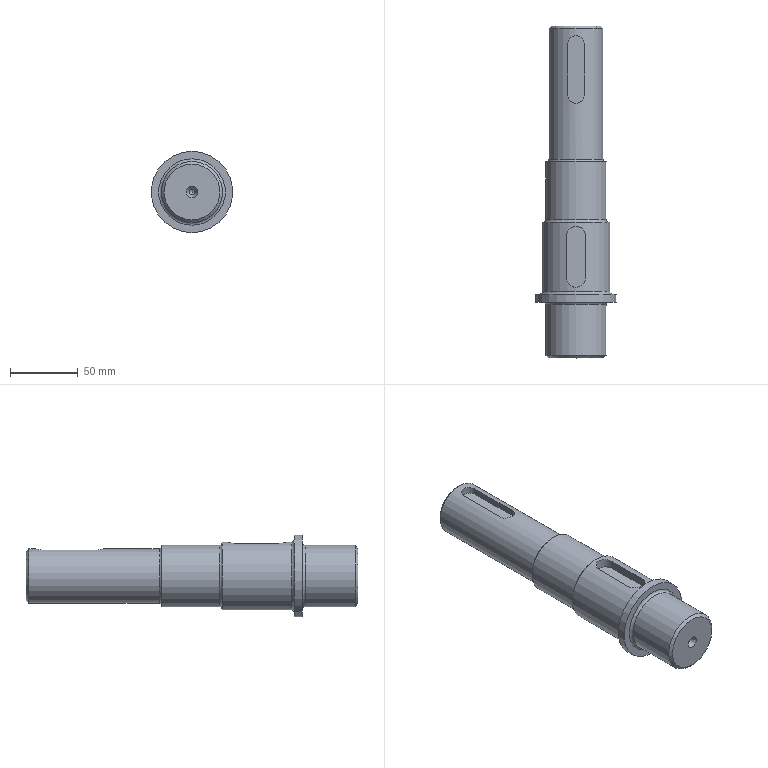Part | NX | features DATUM_CSYS 4, SKETCH 3, EXTRUDE 2, SWP104 1 | 1 solid | 33 faces | box 60 x 244.5 x 60 mm | volume 375385 mm3 | plane 12 | cylinder 11 | cone 6 | torus 4 | commonest cylinder face diameters 4 x2 12 x2 14 x2 45 x2 40 x1 50 x1
STEP:
#1=CARTESIAN_POINT('',(0.,242.5,-20.));
#2=VERTEX_POINT('',#1);
#3=CARTESIAN_POINT('',(0.,242.5,0.));
#4=DIRECTION('',(0.,-1.,0.));
#5=DIRECTION('',(0.,0.,-1.));
#6=AXIS2_PLACEMENT_3D('',#3,#4,#5);
#7=CIRCLE('',#6,20.);
#8=EDGE_CURVE('',#2,#2,#7,.T.);
#9=ORIENTED_EDGE('',*,*,#8,.T.);
#10=EDGE_LOOP('',(#9));
#11=FACE_BOUND('',#10,.T.);
#12=CARTESIAN_POINT('',(0.,146.5,-20.));
#13=VERTEX_POINT('',#12);
#14=CARTESIAN_POINT('',(0.,146.5,0.));
#15=DIRECTION('',(0.,-1.,0.));
#16=DIRECTION('',(0.,0.,-1.));
#17=AXIS2_PLACEMENT_3D('',#14,#15,#16);
#18=CIRCLE('',#17,20.);
#19=EDGE_CURVE('',#13,#13,#18,.T.);
#20=ORIENTED_EDGE('',*,*,#19,.F.);
#21=EDGE_LOOP('',(#20));
#22=FACE_BOUND('',#21,.T.);
#23=CARTESIAN_POINT('',(6.,193.5,19.079));
#24=VERTEX_POINT('',#23);
#25=CARTESIAN_POINT('',(-6.,193.5,19.079));
#26=VERTEX_POINT('',#25);
#27=CARTESIAN_POINT('',(6.,193.5,19.079));
#28=CARTESIAN_POINT('',(6.,191.905,19.079));
#29=CARTESIAN_POINT('',(4.699,188.813,19.55));
#30=CARTESIAN_POINT('',(0.009548,186.844,20.225));
#31=CARTESIAN_POINT('',(-4.702,188.81,19.551));
#32=CARTESIAN_POINT('',(-6.,191.905,19.079));
#33=CARTESIAN_POINT('',(-6.,193.5,19.079));
#34=B_SPLINE_CURVE_WITH_KNOTS('',3,(#27,#28,#29,#30,#31,#32,#33),.UNSPECIFIED.,.F.,.F.,(4,1,1,1,4),(0.,0.004715,0.009431,0.01415,0.01886),.UNSPECIFIED.);
#35=EDGE_CURVE('',#24,#26,#34,.T.);
#36=ORIENTED_EDGE('',*,*,#35,.T.);
#37=CARTESIAN_POINT('',(-6.,231.5,19.079));
#38=VERTEX_POINT('',#37);
#39=CARTESIAN_POINT('',(-6.,122.25,19.079));
#40=DIRECTION('',(0.,-1.,0.));
#41=VECTOR('',#40,1000.);
#42=LINE('',#39,#41);
#43=EDGE_CURVE('',#26,#38,#42,.F.);
#44=ORIENTED_EDGE('',*,*,#43,.T.);
#45=CARTESIAN_POINT('',(6.,231.5,19.079));
#46=VERTEX_POINT('',#45);
#47=CARTESIAN_POINT('',(-6.,231.5,19.079));
#48=CARTESIAN_POINT('',(-6.,233.095,19.079));
#49=CARTESIAN_POINT('',(-4.699,236.187,19.55));
#50=CARTESIAN_POINT('',(-0.009548,238.156,20.225));
#51=CARTESIAN_POINT('',(4.702,236.19,19.551));
#52=CARTESIAN_POINT('',(6.,233.095,19.079));
#53=CARTESIAN_POINT('',(6.,231.5,19.079));
#54=B_SPLINE_CURVE_WITH_KNOTS('',3,(#47,#48,#49,#50,#51,#52,#53),.UNSPECIFIED.,.F.,.F.,(4,1,1,1,4),(0.,0.004715,0.009431,0.01415,0.01886),.UNSPECIFIED.);
#55=EDGE_CURVE('',#38,#46,#54,.T.);
#56=ORIENTED_EDGE('',*,*,#55,.T.);
#57=CARTESIAN_POINT('',(6.,122.25,19.079));
#58=DIRECTION('',(0.,-1.,0.));
#59=VECTOR('',#58,1000.);
#60=LINE('',#57,#59);
#61=EDGE_CURVE('',#46,#24,#60,.T.);
#62=ORIENTED_EDGE('',*,*,#61,.T.);
#63=EDGE_LOOP('',(#36,#44,#56,#62));
#64=FACE_BOUND('',#63,.T.);
#65=CARTESIAN_POINT('',(0.,122.25,0.));
#66=DIRECTION('',(0.,-1.,0.));
#67=DIRECTION('',(0.,0.,-1.));
#68=AXIS2_PLACEMENT_3D('',#65,#66,#67);
#69=CYLINDRICAL_SURFACE('',#68,20.);
#70=ADVANCED_FACE('',(#11,#22,#64),#69,.T.);
#71=CARTESIAN_POINT('',(0.,100.,-25.));
#72=VERTEX_POINT('',#71);
#73=CARTESIAN_POINT('',(0.,100.,0.));
#74=DIRECTION('',(0.,-1.,0.));
#75=DIRECTION('',(0.,0.,-1.));
#76=AXIS2_PLACEMENT_3D('',#73,#74,#75);
#77=CIRCLE('',#76,25.);
#78=EDGE_CURVE('',#72,#72,#77,.T.);
#79=ORIENTED_EDGE('',*,*,#78,.T.);
#80=EDGE_LOOP('',(#79));
#81=FACE_BOUND('',#80,.T.);
#82=CARTESIAN_POINT('',(0.,49.,-25.));
#83=VERTEX_POINT('',#82);
#84=CARTESIAN_POINT('',(0.,49.,0.));
#85=DIRECTION('',(0.,-1.,0.));
#86=DIRECTION('',(0.,0.,-1.));
#87=AXIS2_PLACEMENT_3D('',#84,#85,#86);
#88=CIRCLE('',#87,25.);
#89=EDGE_CURVE('',#83,#83,#88,.T.);
#90=ORIENTED_EDGE('',*,*,#89,.F.);
#91=EDGE_LOOP('',(#90));
#92=FACE_BOUND('',#91,.T.);
#93=CARTESIAN_POINT('',(7.,59.,24.));
#94=VERTEX_POINT('',#93);
#95=CARTESIAN_POINT('',(-7.,59.,24.));
#96=VERTEX_POINT('',#95);
#97=CARTESIAN_POINT('',(7.,59.,24.));
#98=CARTESIAN_POINT('',(7.,57.141,24.));
#99=CARTESIAN_POINT('',(5.483,53.53,24.51));
#100=CARTESIAN_POINT('',(0.01059,51.236,25.245));
#101=CARTESIAN_POINT('',(-5.485,53.527,24.511));
#102=CARTESIAN_POINT('',(-7.,57.14,24.));
#103=CARTESIAN_POINT('',(-7.,59.,24.));
#104=B_SPLINE_CURVE_WITH_KNOTS('',3,(#97,#98,#99,#100,#101,#102,#103),.UNSPECIFIED.,.F.,.F.,(4,1,1,1,4),(0.,0.005497,0.01099,0.01649,0.02199),.UNSPECIFIED.);
#105=EDGE_CURVE('',#94,#96,#104,.T.);
#106=ORIENTED_EDGE('',*,*,#105,.T.);
#107=CARTESIAN_POINT('',(-7.,90.,24.));
#108=VERTEX_POINT('',#107);
#109=CARTESIAN_POINT('',(-7.,122.25,24.));
#110=DIRECTION('',(0.,-1.,0.));
#111=VECTOR('',#110,1000.);
#112=LINE('',#109,#111);
#113=EDGE_CURVE('',#96,#108,#112,.F.);
#114=ORIENTED_EDGE('',*,*,#113,.T.);
#115=CARTESIAN_POINT('',(7.,90.,24.));
#116=VERTEX_POINT('',#115);
#117=CARTESIAN_POINT('',(-7.,90.,24.));
#118=CARTESIAN_POINT('',(-7.,91.859,24.));
#119=CARTESIAN_POINT('',(-5.483,95.47,24.51));
#120=CARTESIAN_POINT('',(-0.01059,97.764,25.245));
#121=CARTESIAN_POINT('',(5.485,95.473,24.511));
#122=CARTESIAN_POINT('',(7.,91.86,24.));
#123=CARTESIAN_POINT('',(7.,90.,24.));
#124=B_SPLINE_CURVE_WITH_KNOTS('',3,(#117,#118,#119,#120,#121,#122,#123),.UNSPECIFIED.,.F.,.F.,(4,1,1,1,4),(0.,0.005497,0.01099,0.01649,0.02199),.UNSPECIFIED.);
#125=EDGE_CURVE('',#108,#116,#124,.T.);
#126=ORIENTED_EDGE('',*,*,#125,.T.);
#127=CARTESIAN_POINT('',(7.,122.25,24.));
#128=DIRECTION('',(0.,-1.,0.));
#129=VECTOR('',#128,1000.);
#130=LINE('',#127,#129);
#131=EDGE_CURVE('',#116,#94,#130,.T.);
#132=ORIENTED_EDGE('',*,*,#131,.T.);
#133=EDGE_LOOP('',(#106,#114,#126,#132));
#134=FACE_BOUND('',#133,.T.);
#135=CARTESIAN_POINT('',(0.,122.25,0.));
#136=DIRECTION('',(0.,-1.,0.));
#137=DIRECTION('',(0.,0.,-1.));
#138=AXIS2_PLACEMENT_3D('',#135,#136,#137);
#139=CYLINDRICAL_SURFACE('',#138,25.);
#140=ADVANCED_FACE('',(#81,#92,#134),#139,.T.);
#141=CARTESIAN_POINT('',(0.,0.,-4.309));
#142=VERTEX_POINT('',#141);
#143=CARTESIAN_POINT('',(0.,0.,0.));
#144=DIRECTION('',(0.,-1.,0.));
#145=DIRECTION('',(0.,0.,-1.));
#146=AXIS2_PLACEMENT_3D('',#143,#144,#145);
#147=CIRCLE('',#146,4.309);
#148=EDGE_CURVE('',#142,#142,#147,.T.);
#149=ORIENTED_EDGE('',*,*,#148,.F.);
#150=EDGE_LOOP('',(#149));
#151=FACE_BOUND('',#150,.T.);
#152=CARTESIAN_POINT('',(0.,0.,-20.5));
#153=VERTEX_POINT('',#152);
#154=CARTESIAN_POINT('',(0.,0.,0.));
#155=DIRECTION('',(0.,-1.,0.));
#156=DIRECTION('',(0.,0.,-1.));
#157=AXIS2_PLACEMENT_3D('',#154,#155,#156);
#158=CIRCLE('',#157,20.5);
#159=EDGE_CURVE('',#153,#153,#158,.T.);
#160=ORIENTED_EDGE('',*,*,#159,.T.);
#161=EDGE_LOOP('',(#160));
#162=FACE_BOUND('',#161,.T.);
#163=CARTESIAN_POINT('',(0.,0.,20.5));
#164=DIRECTION('',(0.,1.,0.));
#165=DIRECTION('',(0.,0.,1.));
#166=AXIS2_PLACEMENT_3D('',#163,#164,#165);
#167=PLANE('',#166);
#168=ADVANCED_FACE('',(#151,#162),#167,.F.);
#169=CARTESIAN_POINT('',(0.,4.,-2.));
#170=VERTEX_POINT('',#169);
#171=CARTESIAN_POINT('',(0.,4.,0.));
#172=DIRECTION('',(0.,-1.,0.));
#173=DIRECTION('',(0.,0.,-1.));
#174=AXIS2_PLACEMENT_3D('',#171,#172,#173);
#175=CIRCLE('',#174,2.);
#176=EDGE_CURVE('',#170,#170,#175,.T.);
#177=ORIENTED_EDGE('',*,*,#176,.F.);
#178=EDGE_LOOP('',(#177));
#179=FACE_BOUND('',#178,.T.);
#180=ORIENTED_EDGE('',*,*,#148,.T.);
#181=EDGE_LOOP('',(#180));
#182=FACE_BOUND('',#181,.T.);
#183=CARTESIAN_POINT('',(0.,0.,0.));
#184=DIRECTION('',(0.,-1.,0.));
#185=DIRECTION('',(0.,0.,-1.));
#186=AXIS2_PLACEMENT_3D('',#183,#184,#185);
#187=CONICAL_SURFACE('',#186,4.309,0.5236);
#188=ADVANCED_FACE('',(#179,#182),#187,.F.);
#189=CARTESIAN_POINT('',(0.,8.,-2.));
#190=VERTEX_POINT('',#189);
#191=CARTESIAN_POINT('',(0.,8.,0.));
#192=DIRECTION('',(0.,-1.,0.));
#193=DIRECTION('',(0.,0.,-1.));
#194=AXIS2_PLACEMENT_3D('',#191,#192,#193);
#195=CIRCLE('',#194,2.);
#196=EDGE_CURVE('',#190,#190,#195,.T.);
#197=ORIENTED_EDGE('',*,*,#196,.F.);
#198=EDGE_LOOP('',(#197));
#199=FACE_BOUND('',#198,.T.);
#200=ORIENTED_EDGE('',*,*,#176,.T.);
#201=EDGE_LOOP('',(#200));
#202=FACE_BOUND('',#201,.T.);
#203=CARTESIAN_POINT('',(0.,122.25,0.));
#204=DIRECTION('',(0.,-1.,0.));
#205=DIRECTION('',(0.,0.,-1.));
#206=AXIS2_PLACEMENT_3D('',#203,#204,#205);
#207=CYLINDRICAL_SURFACE('',#206,2.);
#208=ADVANCED_FACE('',(#199,#202),#207,.F.);
#209=CARTESIAN_POINT('',(0.,9.155,0.));
#210=VERTEX_POINT('',#209);
#211=VERTEX_LOOP('',#210);
#212=FACE_BOUND('',#211,.T.);
#213=ORIENTED_EDGE('',*,*,#196,.T.);
#214=EDGE_LOOP('',(#213));
#215=FACE_BOUND('',#214,.T.);
#216=CARTESIAN_POINT('',(0.,8.,0.));
#217=DIRECTION('',(0.,-1.,0.));
#218=DIRECTION('',(0.,0.,-1.));
#219=AXIS2_PLACEMENT_3D('',#216,#217,#218);
#220=CONICAL_SURFACE('',#219,2.,1.047);
#221=ADVANCED_FACE('',(#212,#215),#220,.F.);
#222=CARTESIAN_POINT('',(0.,236.5,-2.));
#223=VERTEX_POINT('',#222);
#224=CARTESIAN_POINT('',(0.,236.5,0.));
#225=DIRECTION('',(0.,-1.,0.));
#226=DIRECTION('',(0.,0.,-1.));
#227=AXIS2_PLACEMENT_3D('',#224,#225,#226);
#228=CIRCLE('',#227,2.);
#229=EDGE_CURVE('',#223,#223,#228,.T.);
#230=ORIENTED_EDGE('',*,*,#229,.F.);
#231=EDGE_LOOP('',(#230));
#232=FACE_BOUND('',#231,.T.);
#233=CARTESIAN_POINT('',(0.,235.345,0.));
#234=VERTEX_POINT('',#233);
#235=VERTEX_LOOP('',#234);
#236=FACE_BOUND('',#235,.T.);
#237=CARTESIAN_POINT('',(0.,235.345,0.));
#238=DIRECTION('',(0.,1.,0.));
#239=DIRECTION('',(0.,0.,1.));
#240=AXIS2_PLACEMENT_3D('',#237,#238,#239);
#241=CONICAL_SURFACE('',#240,0.,1.047);
#242=ADVANCED_FACE('',(#232,#236),#241,.F.);
#243=CARTESIAN_POINT('',(0.,240.5,-2.));
#244=VERTEX_POINT('',#243);
#245=CARTESIAN_POINT('',(0.,240.5,0.));
#246=DIRECTION('',(0.,-1.,0.));
#247=DIRECTION('',(0.,0.,-1.));
#248=AXIS2_PLACEMENT_3D('',#245,#246,#247);
#249=CIRCLE('',#248,2.);
#250=EDGE_CURVE('',#244,#244,#249,.T.);
#251=ORIENTED_EDGE('',*,*,#250,.F.);
#252=EDGE_LOOP('',(#251));
#253=FACE_BOUND('',#252,.T.);
#254=ORIENTED_EDGE('',*,*,#229,.T.);
#255=EDGE_LOOP('',(#254));
#256=FACE_BOUND('',#255,.T.);
#257=CARTESIAN_POINT('',(0.,122.25,0.));
#258=DIRECTION('',(0.,-1.,0.));
#259=DIRECTION('',(0.,0.,-1.));
#260=AXIS2_PLACEMENT_3D('',#257,#258,#259);
#261=CYLINDRICAL_SURFACE('',#260,2.);
#262=ADVANCED_FACE('',(#253,#256),#261,.F.);
#263=CARTESIAN_POINT('',(0.,244.5,-4.309));
#264=VERTEX_POINT('',#263);
#265=CARTESIAN_POINT('',(0.,244.5,0.));
#266=DIRECTION('',(0.,-1.,0.));
#267=DIRECTION('',(0.,0.,-1.));
#268=AXIS2_PLACEMENT_3D('',#265,#266,#267);
#269=CIRCLE('',#268,4.309);
#270=EDGE_CURVE('',#264,#264,#269,.T.);
#271=ORIENTED_EDGE('',*,*,#270,.F.);
#272=EDGE_LOOP('',(#271));
#273=FACE_BOUND('',#272,.T.);
#274=ORIENTED_EDGE('',*,*,#250,.T.);
#275=EDGE_LOOP('',(#274));
#276=FACE_BOUND('',#275,.T.);
#277=CARTESIAN_POINT('',(0.,240.5,0.));
#278=DIRECTION('',(0.,1.,0.));
#279=DIRECTION('',(0.,0.,1.));
#280=AXIS2_PLACEMENT_3D('',#277,#278,#279);
#281=CONICAL_SURFACE('',#280,2.,0.5236);
#282=ADVANCED_FACE('',(#273,#276),#281,.F.);
#283=CARTESIAN_POINT('',(0.,244.5,-18.));
#284=VERTEX_POINT('',#283);
#285=CARTESIAN_POINT('',(0.,244.5,0.));
#286=DIRECTION('',(0.,-1.,0.));
#287=DIRECTION('',(0.,0.,-1.));
#288=AXIS2_PLACEMENT_3D('',#285,#286,#287);
#289=CIRCLE('',#288,18.);
#290=EDGE_CURVE('',#284,#284,#289,.T.);
#291=ORIENTED_EDGE('',*,*,#290,.F.);
#292=EDGE_LOOP('',(#291));
#293=FACE_BOUND('',#292,.T.);
#294=ORIENTED_EDGE('',*,*,#270,.T.);
#295=EDGE_LOOP('',(#294));
#296=FACE_BOUND('',#295,.T.);
#297=CARTESIAN_POINT('',(0.,244.5,4.309));
#298=DIRECTION('',(0.,-1.,0.));
#299=DIRECTION('',(0.,0.,-1.));
#300=AXIS2_PLACEMENT_3D('',#297,#298,#299);
#301=PLANE('',#300);
#302=ADVANCED_FACE('',(#293,#296),#301,.F.);
#303=ORIENTED_EDGE('',*,*,#8,.F.);
#304=EDGE_LOOP('',(#303));
#305=FACE_BOUND('',#304,.T.);
#306=ORIENTED_EDGE('',*,*,#290,.T.);
#307=EDGE_LOOP('',(#306));
#308=FACE_BOUND('',#307,.T.);
#309=CARTESIAN_POINT('',(0.,244.5,0.));
#310=DIRECTION('',(0.,-1.,0.));
#311=DIRECTION('',(0.,0.,-1.));
#312=AXIS2_PLACEMENT_3D('',#309,#310,#311);
#313=CONICAL_SURFACE('',#312,18.,0.7854);
#314=ADVANCED_FACE('',(#305,#308),#313,.T.);
#315=CARTESIAN_POINT('',(0.,144.5,-22.));
#316=VERTEX_POINT('',#315);
#317=CARTESIAN_POINT('',(0.,144.5,0.));
#318=DIRECTION('',(0.,-1.,0.));
#319=DIRECTION('',(0.,0.,-1.));
#320=AXIS2_PLACEMENT_3D('',#317,#318,#319);
#321=CIRCLE('',#320,22.);
#322=EDGE_CURVE('',#316,#316,#321,.T.);
#323=ORIENTED_EDGE('',*,*,#322,.F.);
#324=EDGE_LOOP('',(#323));
#325=FACE_BOUND('',#324,.T.);
#326=ORIENTED_EDGE('',*,*,#19,.T.);
#327=EDGE_LOOP('',(#326));
#328=FACE_BOUND('',#327,.T.);
#329=CARTESIAN_POINT('',(0.,146.5,0.));
#330=DIRECTION('',(0.,-1.,0.));
#331=DIRECTION('',(0.,0.,-1.));
#332=AXIS2_PLACEMENT_3D('',#329,#330,#331);
#333=TOROIDAL_SURFACE('',#332,22.,2.);
#334=ADVANCED_FACE('',(#325,#328),#333,.F.);
#335=CARTESIAN_POINT('',(0.,144.5,-22.5));
#336=VERTEX_POINT('',#335);
#337=CARTESIAN_POINT('',(0.,144.5,0.));
#338=DIRECTION('',(0.,-1.,0.));
#339=DIRECTION('',(0.,0.,-1.));
#340=AXIS2_PLACEMENT_3D('',#337,#338,#339);
#341=CIRCLE('',#340,22.5);
#342=EDGE_CURVE('',#336,#336,#341,.T.);
#343=ORIENTED_EDGE('',*,*,#342,.F.);
#344=EDGE_LOOP('',(#343));
#345=FACE_BOUND('',#344,.T.);
#346=ORIENTED_EDGE('',*,*,#322,.T.);
#347=EDGE_LOOP('',(#346));
#348=FACE_BOUND('',#347,.T.);
#349=CARTESIAN_POINT('',(0.,144.5,22.));
#350=DIRECTION('',(0.,-1.,0.));
#351=DIRECTION('',(0.,0.,-1.));
#352=AXIS2_PLACEMENT_3D('',#349,#350,#351);
#353=PLANE('',#352);
#354=ADVANCED_FACE('',(#345,#348),#353,.F.);
#355=CARTESIAN_POINT('',(0.,102.,-22.5));
#356=VERTEX_POINT('',#355);
#357=CARTESIAN_POINT('',(0.,102.,0.));
#358=DIRECTION('',(0.,-1.,0.));
#359=DIRECTION('',(0.,0.,-1.));
#360=AXIS2_PLACEMENT_3D('',#357,#358,#359);
#361=CIRCLE('',#360,22.5);
#362=EDGE_CURVE('',#356,#356,#361,.T.);
#363=ORIENTED_EDGE('',*,*,#362,.F.);
#364=EDGE_LOOP('',(#363));
#365=FACE_BOUND('',#364,.T.);
#366=ORIENTED_EDGE('',*,*,#342,.T.);
#367=EDGE_LOOP('',(#366));
#368=FACE_BOUND('',#367,.T.);
#369=CARTESIAN_POINT('',(0.,122.25,0.));
#370=DIRECTION('',(0.,-1.,0.));
#371=DIRECTION('',(0.,0.,-1.));
#372=AXIS2_PLACEMENT_3D('',#369,#370,#371);
#373=CYLINDRICAL_SURFACE('',#372,22.5);
#374=ADVANCED_FACE('',(#365,#368),#373,.T.);
#375=CARTESIAN_POINT('',(0.,100.,-24.5));
#376=VERTEX_POINT('',#375);
#377=CARTESIAN_POINT('',(0.,100.,0.));
#378=DIRECTION('',(0.,-1.,0.));
#379=DIRECTION('',(0.,0.,-1.));
#380=AXIS2_PLACEMENT_3D('',#377,#378,#379);
#381=CIRCLE('',#380,24.5);
#382=EDGE_CURVE('',#376,#376,#381,.T.);
#383=ORIENTED_EDGE('',*,*,#382,.F.);
#384=EDGE_LOOP('',(#383));
#385=FACE_BOUND('',#384,.T.);
#386=ORIENTED_EDGE('',*,*,#362,.T.);
#387=EDGE_LOOP('',(#386));
#388=FACE_BOUND('',#387,.T.);
#389=CARTESIAN_POINT('',(0.,102.,0.));
#390=DIRECTION('',(0.,-1.,0.));
#391=DIRECTION('',(0.,0.,-1.));
#392=AXIS2_PLACEMENT_3D('',#389,#390,#391);
#393=TOROIDAL_SURFACE('',#392,24.5,2.);
#394=ADVANCED_FACE('',(#385,#388),#393,.F.);
#395=ORIENTED_EDGE('',*,*,#78,.F.);
#396=EDGE_LOOP('',(#395));
#397=FACE_BOUND('',#396,.T.);
#398=ORIENTED_EDGE('',*,*,#382,.T.);
#399=EDGE_LOOP('',(#398));
#400=FACE_BOUND('',#399,.T.);
#401=CARTESIAN_POINT('',(0.,100.,24.5));
#402=DIRECTION('',(0.,-1.,0.));
#403=DIRECTION('',(0.,0.,-1.));
#404=AXIS2_PLACEMENT_3D('',#401,#402,#403);
#405=PLANE('',#404);
#406=ADVANCED_FACE('',(#397,#400),#405,.F.);
#407=CARTESIAN_POINT('',(0.,47.,-27.));
#408=VERTEX_POINT('',#407);
#409=CARTESIAN_POINT('',(0.,47.,0.));
#410=DIRECTION('',(0.,-1.,0.));
#411=DIRECTION('',(0.,0.,-1.));
#412=AXIS2_PLACEMENT_3D('',#409,#410,#411);
#413=CIRCLE('',#412,27.);
#414=EDGE_CURVE('',#408,#408,#413,.T.);
#415=ORIENTED_EDGE('',*,*,#414,.F.);
#416=EDGE_LOOP('',(#415));
#417=FACE_BOUND('',#416,.T.);
#418=ORIENTED_EDGE('',*,*,#89,.T.);
#419=EDGE_LOOP('',(#418));
#420=FACE_BOUND('',#419,.T.);
#421=CARTESIAN_POINT('',(0.,49.,0.));
#422=DIRECTION('',(0.,-1.,0.));
#423=DIRECTION('',(0.,0.,-1.));
#424=AXIS2_PLACEMENT_3D('',#421,#422,#423);
#425=TOROIDAL_SURFACE('',#424,27.,2.);
#426=ADVANCED_FACE('',(#417,#420),#425,.F.);
#427=CARTESIAN_POINT('',(0.,47.,-30.));
#428=VERTEX_POINT('',#427);
#429=CARTESIAN_POINT('',(0.,47.,0.));
#430=DIRECTION('',(0.,-1.,0.));
#431=DIRECTION('',(0.,0.,-1.));
#432=AXIS2_PLACEMENT_3D('',#429,#430,#431);
#433=CIRCLE('',#432,30.);
#434=EDGE_CURVE('',#428,#428,#433,.T.);
#435=ORIENTED_EDGE('',*,*,#434,.F.);
#436=EDGE_LOOP('',(#435));
#437=FACE_BOUND('',#436,.T.);
#438=ORIENTED_EDGE('',*,*,#414,.T.);
#439=EDGE_LOOP('',(#438));
#440=FACE_BOUND('',#439,.T.);
#441=CARTESIAN_POINT('',(0.,47.,27.));
#442=DIRECTION('',(0.,-1.,0.));
#443=DIRECTION('',(0.,0.,-1.));
#444=AXIS2_PLACEMENT_3D('',#441,#442,#443);
#445=PLANE('',#444);
#446=ADVANCED_FACE('',(#437,#440),#445,.F.);
#447=CARTESIAN_POINT('',(0.,41.,-30.));
#448=VERTEX_POINT('',#447);
#449=CARTESIAN_POINT('',(0.,41.,0.));
#450=DIRECTION('',(0.,-1.,0.));
#451=DIRECTION('',(0.,0.,-1.));
#452=AXIS2_PLACEMENT_3D('',#449,#450,#451);
#453=CIRCLE('',#452,30.);
#454=EDGE_CURVE('',#448,#448,#453,.T.);
#455=ORIENTED_EDGE('',*,*,#454,.F.);
#456=EDGE_LOOP('',(#455));
#457=FACE_BOUND('',#456,.T.);
#458=ORIENTED_EDGE('',*,*,#434,.T.);
#459=EDGE_LOOP('',(#458));
#460=FACE_BOUND('',#459,.T.);
#461=CARTESIAN_POINT('',(0.,122.25,0.));
#462=DIRECTION('',(0.,-1.,0.));
#463=DIRECTION('',(0.,0.,-1.));
#464=AXIS2_PLACEMENT_3D('',#461,#462,#463);
#465=CYLINDRICAL_SURFACE('',#464,30.);
#466=ADVANCED_FACE('',(#457,#460),#465,.T.);
#467=CARTESIAN_POINT('',(0.,41.,-24.5));
#468=VERTEX_POINT('',#467);
#469=CARTESIAN_POINT('',(0.,41.,0.));
#470=DIRECTION('',(0.,-1.,0.));
#471=DIRECTION('',(0.,0.,-1.));
#472=AXIS2_PLACEMENT_3D('',#469,#470,#471);
#473=CIRCLE('',#472,24.5);
#474=EDGE_CURVE('',#468,#468,#473,.T.);
#475=ORIENTED_EDGE('',*,*,#474,.F.);
#476=EDGE_LOOP('',(#475));
#477=FACE_BOUND('',#476,.T.);
#478=ORIENTED_EDGE('',*,*,#454,.T.);
#479=EDGE_LOOP('',(#478));
#480=FACE_BOUND('',#479,.T.);
#481=CARTESIAN_POINT('',(0.,41.,30.));
#482=DIRECTION('',(0.,1.,0.));
#483=DIRECTION('',(0.,0.,1.));
#484=AXIS2_PLACEMENT_3D('',#481,#482,#483);
#485=PLANE('',#484);
#486=ADVANCED_FACE('',(#477,#480),#485,.F.);
#487=CARTESIAN_POINT('',(0.,39.,-22.5));
#488=VERTEX_POINT('',#487);
#489=CARTESIAN_POINT('',(0.,39.,0.));
#490=DIRECTION('',(0.,-1.,0.));
#491=DIRECTION('',(0.,0.,-1.));
#492=AXIS2_PLACEMENT_3D('',#489,#490,#491);
#493=CIRCLE('',#492,22.5);
#494=EDGE_CURVE('',#488,#488,#493,.T.);
#495=ORIENTED_EDGE('',*,*,#494,.F.);
#496=EDGE_LOOP('',(#495));
#497=FACE_BOUND('',#496,.T.);
#498=ORIENTED_EDGE('',*,*,#474,.T.);
#499=EDGE_LOOP('',(#498));
#500=FACE_BOUND('',#499,.T.);
#501=CARTESIAN_POINT('',(0.,39.,0.));
#502=DIRECTION('',(0.,-1.,0.));
#503=DIRECTION('',(0.,0.,-1.));
#504=AXIS2_PLACEMENT_3D('',#501,#502,#503);
#505=TOROIDAL_SURFACE('',#504,24.5,2.);
#506=ADVANCED_FACE('',(#497,#500),#505,.F.);
#507=CARTESIAN_POINT('',(0.,2.,-22.5));
#508=VERTEX_POINT('',#507);
#509=CARTESIAN_POINT('',(0.,2.,0.));
#510=DIRECTION('',(0.,-1.,0.));
#511=DIRECTION('',(0.,0.,-1.));
#512=AXIS2_PLACEMENT_3D('',#509,#510,#511);
#513=CIRCLE('',#512,22.5);
#514=EDGE_CURVE('',#508,#508,#513,.T.);
#515=ORIENTED_EDGE('',*,*,#514,.F.);
#516=EDGE_LOOP('',(#515));
#517=FACE_BOUND('',#516,.T.);
#518=ORIENTED_EDGE('',*,*,#494,.T.);
#519=EDGE_LOOP('',(#518));
#520=FACE_BOUND('',#519,.T.);
#521=CARTESIAN_POINT('',(0.,122.25,0.));
#522=DIRECTION('',(0.,-1.,0.));
#523=DIRECTION('',(0.,0.,-1.));
#524=AXIS2_PLACEMENT_3D('',#521,#522,#523);
#525=CYLINDRICAL_SURFACE('',#524,22.5);
#526=ADVANCED_FACE('',(#517,#520),#525,.T.);
#527=ORIENTED_EDGE('',*,*,#159,.F.);
#528=EDGE_LOOP('',(#527));
#529=FACE_BOUND('',#528,.T.);
#530=ORIENTED_EDGE('',*,*,#514,.T.);
#531=EDGE_LOOP('',(#530));
#532=FACE_BOUND('',#531,.T.);
#533=CARTESIAN_POINT('',(0.,2.,0.));
#534=DIRECTION('',(0.,1.,0.));
#535=DIRECTION('',(0.,0.,1.));
#536=AXIS2_PLACEMENT_3D('',#533,#534,#535);
#537=CONICAL_SURFACE('',#536,22.5,0.7854);
#538=ADVANCED_FACE('',(#529,#532),#537,.T.);
#539=CARTESIAN_POINT('',(7.,59.,18.));
#540=VERTEX_POINT('',#539);
#541=CARTESIAN_POINT('',(7.,59.,247.5));
#542=DIRECTION('',(0.,0.,-1.));
#543=VECTOR('',#542,1000.);
#544=LINE('',#541,#543);
#545=EDGE_CURVE('',#540,#94,#544,.F.);
#546=ORIENTED_EDGE('',*,*,#545,.F.);
#547=CARTESIAN_POINT('',(-7.,59.,18.));
#548=VERTEX_POINT('',#547);
#549=CARTESIAN_POINT('',(0.,59.,18.));
#550=DIRECTION('',(0.,0.,1.));
#551=DIRECTION('',(1.,0.,0.));
#552=AXIS2_PLACEMENT_3D('',#549,#550,#551);
#553=CIRCLE('',#552,7.);
#554=EDGE_CURVE('',#540,#548,#553,.F.);
#555=ORIENTED_EDGE('',*,*,#554,.T.);
#556=CARTESIAN_POINT('',(-7.,59.,247.5));
#557=DIRECTION('',(0.,0.,-1.));
#558=VECTOR('',#557,1000.);
#559=LINE('',#556,#558);
#560=EDGE_CURVE('',#548,#96,#559,.F.);
#561=ORIENTED_EDGE('',*,*,#560,.T.);
#562=ORIENTED_EDGE('',*,*,#105,.F.);
#563=EDGE_LOOP('',(#546,#555,#561,#562));
#564=FACE_BOUND('',#563,.T.);
#565=CARTESIAN_POINT('',(0.,59.,247.5));
#566=DIRECTION('',(0.,0.,-1.));
#567=DIRECTION('',(-1.,0.,0.));
#568=AXIS2_PLACEMENT_3D('',#565,#566,#567);
#569=CYLINDRICAL_SURFACE('',#568,7.);
#570=ADVANCED_FACE('',(#564),#569,.F.);
#571=CARTESIAN_POINT('',(-7.,90.,18.));
#572=VERTEX_POINT('',#571);
#573=CARTESIAN_POINT('',(-7.,90.,18.));
#574=DIRECTION('',(0.,-1.,0.));
#575=VECTOR('',#574,1000.);
#576=LINE('',#573,#575);
#577=EDGE_CURVE('',#548,#572,#576,.F.);
#578=ORIENTED_EDGE('',*,*,#577,.F.);
#579=ORIENTED_EDGE('',*,*,#554,.F.);
#580=CARTESIAN_POINT('',(7.,90.,18.));
#581=VERTEX_POINT('',#580);
#582=CARTESIAN_POINT('',(7.,59.,18.));
#583=DIRECTION('',(0.,1.,0.));
#584=VECTOR('',#583,1000.);
#585=LINE('',#582,#584);
#586=EDGE_CURVE('',#581,#540,#585,.F.);
#587=ORIENTED_EDGE('',*,*,#586,.F.);
#588=CARTESIAN_POINT('',(0.,90.,18.));
#589=DIRECTION('',(0.,0.,1.));
#590=DIRECTION('',(1.,0.,0.));
#591=AXIS2_PLACEMENT_3D('',#588,#589,#590);
#592=CIRCLE('',#591,7.);
#593=EDGE_CURVE('',#572,#581,#592,.F.);
#594=ORIENTED_EDGE('',*,*,#593,.F.);
#595=EDGE_LOOP('',(#578,#579,#587,#594));
#596=FACE_BOUND('',#595,.T.);
#597=CARTESIAN_POINT('',(0.,59.,18.));
#598=DIRECTION('',(0.,0.,1.));
#599=DIRECTION('',(1.,0.,0.));
#600=AXIS2_PLACEMENT_3D('',#597,#598,#599);
#601=PLANE('',#600);
#602=ADVANCED_FACE('',(#596),#601,.T.);
#603=CARTESIAN_POINT('',(7.,90.,247.5));
#604=DIRECTION('',(0.,0.,-1.));
#605=VECTOR('',#604,1000.);
#606=LINE('',#603,#605);
#607=EDGE_CURVE('',#581,#116,#606,.F.);
#608=ORIENTED_EDGE('',*,*,#607,.F.);
#609=ORIENTED_EDGE('',*,*,#586,.T.);
#610=ORIENTED_EDGE('',*,*,#545,.T.);
#611=ORIENTED_EDGE('',*,*,#131,.F.);
#612=EDGE_LOOP('',(#608,#609,#610,#611));
#613=FACE_BOUND('',#612,.T.);
#614=CARTESIAN_POINT('',(7.,59.,247.5));
#615=DIRECTION('',(-1.,0.,0.));
#616=DIRECTION('',(0.,-1.,0.));
#617=AXIS2_PLACEMENT_3D('',#614,#615,#616);
#618=PLANE('',#617);
#619=ADVANCED_FACE('',(#613),#618,.T.);
#620=ORIENTED_EDGE('',*,*,#560,.F.);
#621=ORIENTED_EDGE('',*,*,#577,.T.);
#622=CARTESIAN_POINT('',(-7.,90.,247.5));
#623=DIRECTION('',(0.,0.,-1.));
#624=VECTOR('',#623,1000.);
#625=LINE('',#622,#624);
#626=EDGE_CURVE('',#572,#108,#625,.F.);
#627=ORIENTED_EDGE('',*,*,#626,.T.);
#628=ORIENTED_EDGE('',*,*,#113,.F.);
#629=EDGE_LOOP('',(#620,#621,#627,#628));
#630=FACE_BOUND('',#629,.T.);
#631=CARTESIAN_POINT('',(-7.,90.,247.5));
#632=DIRECTION('',(1.,0.,0.));
#633=DIRECTION('',(0.,1.,0.));
#634=AXIS2_PLACEMENT_3D('',#631,#632,#633);
#635=PLANE('',#634);
#636=ADVANCED_FACE('',(#630),#635,.T.);
#637=ORIENTED_EDGE('',*,*,#626,.F.);
#638=ORIENTED_EDGE('',*,*,#593,.T.);
#639=ORIENTED_EDGE('',*,*,#607,.T.);
#640=ORIENTED_EDGE('',*,*,#125,.F.);
#641=EDGE_LOOP('',(#637,#638,#639,#640));
#642=FACE_BOUND('',#641,.T.);
#643=CARTESIAN_POINT('',(0.,90.,247.5));
#644=DIRECTION('',(0.,0.,-1.));
#645=DIRECTION('',(-1.,0.,0.));
#646=AXIS2_PLACEMENT_3D('',#643,#644,#645);
#647=CYLINDRICAL_SURFACE('',#646,7.);
#648=ADVANCED_FACE('',(#642),#647,.F.);
#649=CARTESIAN_POINT('',(6.,193.5,14.5));
#650=VERTEX_POINT('',#649);
#651=CARTESIAN_POINT('',(6.,193.5,198.));
#652=DIRECTION('',(0.,0.,-1.));
#653=VECTOR('',#652,1000.);
#654=LINE('',#651,#653);
#655=EDGE_CURVE('',#650,#24,#654,.F.);
#656=ORIENTED_EDGE('',*,*,#655,.F.);
#657=CARTESIAN_POINT('',(-6.,193.5,14.5));
#658=VERTEX_POINT('',#657);
#659=CARTESIAN_POINT('',(0.,193.5,14.5));
#660=DIRECTION('',(0.,0.,1.));
#661=DIRECTION('',(1.,0.,0.));
#662=AXIS2_PLACEMENT_3D('',#659,#660,#661);
#663=CIRCLE('',#662,6.);
#664=EDGE_CURVE('',#650,#658,#663,.F.);
#665=ORIENTED_EDGE('',*,*,#664,.T.);
#666=CARTESIAN_POINT('',(-6.,193.5,198.));
#667=DIRECTION('',(0.,0.,-1.));
#668=VECTOR('',#667,1000.);
#669=LINE('',#666,#668);
#670=EDGE_CURVE('',#658,#26,#669,.F.);
#671=ORIENTED_EDGE('',*,*,#670,.T.);
#672=ORIENTED_EDGE('',*,*,#35,.F.);
#673=EDGE_LOOP('',(#656,#665,#671,#672));
#674=FACE_BOUND('',#673,.T.);
#675=CARTESIAN_POINT('',(0.,193.5,198.));
#676=DIRECTION('',(0.,0.,-1.));
#677=DIRECTION('',(-1.,0.,0.));
#678=AXIS2_PLACEMENT_3D('',#675,#676,#677);
#679=CYLINDRICAL_SURFACE('',#678,6.);
#680=ADVANCED_FACE('',(#674),#679,.F.);
#681=CARTESIAN_POINT('',(-6.,231.5,14.5));
#682=VERTEX_POINT('',#681);
#683=CARTESIAN_POINT('',(-6.,231.5,14.5));
#684=DIRECTION('',(0.,-1.,0.));
#685=VECTOR('',#684,1000.);
#686=LINE('',#683,#685);
#687=EDGE_CURVE('',#658,#682,#686,.F.);
#688=ORIENTED_EDGE('',*,*,#687,.F.);
#689=ORIENTED_EDGE('',*,*,#664,.F.);
#690=CARTESIAN_POINT('',(6.,231.5,14.5));
#691=VERTEX_POINT('',#690);
#692=CARTESIAN_POINT('',(6.,193.5,14.5));
#693=DIRECTION('',(0.,1.,0.));
#694=VECTOR('',#693,1000.);
#695=LINE('',#692,#694);
#696=EDGE_CURVE('',#691,#650,#695,.F.);
#697=ORIENTED_EDGE('',*,*,#696,.F.);
#698=CARTESIAN_POINT('',(0.,231.5,14.5));
#699=DIRECTION('',(0.,0.,1.));
#700=DIRECTION('',(1.,0.,0.));
#701=AXIS2_PLACEMENT_3D('',#698,#699,#700);
#702=CIRCLE('',#701,6.);
#703=EDGE_CURVE('',#682,#691,#702,.F.);
#704=ORIENTED_EDGE('',*,*,#703,.F.);
#705=EDGE_LOOP('',(#688,#689,#697,#704));
#706=FACE_BOUND('',#705,.T.);
#707=CARTESIAN_POINT('',(0.,193.5,14.5));
#708=DIRECTION('',(0.,0.,1.));
#709=DIRECTION('',(1.,0.,0.));
#710=AXIS2_PLACEMENT_3D('',#707,#708,#709);
#711=PLANE('',#710);
#712=ADVANCED_FACE('',(#706),#711,.T.);
#713=CARTESIAN_POINT('',(6.,231.5,198.));
#714=DIRECTION('',(0.,0.,-1.));
#715=VECTOR('',#714,1000.);
#716=LINE('',#713,#715);
#717=EDGE_CURVE('',#691,#46,#716,.F.);
#718=ORIENTED_EDGE('',*,*,#717,.F.);
#719=ORIENTED_EDGE('',*,*,#696,.T.);
#720=ORIENTED_EDGE('',*,*,#655,.T.);
#721=ORIENTED_EDGE('',*,*,#61,.F.);
#722=EDGE_LOOP('',(#718,#719,#720,#721));
#723=FACE_BOUND('',#722,.T.);
#724=CARTESIAN_POINT('',(6.,193.5,198.));
#725=DIRECTION('',(-1.,0.,0.));
#726=DIRECTION('',(0.,-1.,0.));
#727=AXIS2_PLACEMENT_3D('',#724,#725,#726);
#728=PLANE('',#727);
#729=ADVANCED_FACE('',(#723),#728,.T.);
#730=ORIENTED_EDGE('',*,*,#670,.F.);
#731=ORIENTED_EDGE('',*,*,#687,.T.);
#732=CARTESIAN_POINT('',(-6.,231.5,198.));
#733=DIRECTION('',(0.,0.,-1.));
#734=VECTOR('',#733,1000.);
#735=LINE('',#732,#734);
#736=EDGE_CURVE('',#682,#38,#735,.F.);
#737=ORIENTED_EDGE('',*,*,#736,.T.);
#738=ORIENTED_EDGE('',*,*,#43,.F.);
#739=EDGE_LOOP('',(#730,#731,#737,#738));
#740=FACE_BOUND('',#739,.T.);
#741=CARTESIAN_POINT('',(-6.,231.5,198.));
#742=DIRECTION('',(1.,0.,0.));
#743=DIRECTION('',(0.,1.,0.));
#744=AXIS2_PLACEMENT_3D('',#741,#742,#743);
#745=PLANE('',#744);
#746=ADVANCED_FACE('',(#740),#745,.T.);
#747=ORIENTED_EDGE('',*,*,#736,.F.);
#748=ORIENTED_EDGE('',*,*,#703,.T.);
#749=ORIENTED_EDGE('',*,*,#717,.T.);
#750=ORIENTED_EDGE('',*,*,#55,.F.);
#751=EDGE_LOOP('',(#747,#748,#749,#750));
#752=FACE_BOUND('',#751,.T.);
#753=CARTESIAN_POINT('',(0.,231.5,198.));
#754=DIRECTION('',(0.,0.,-1.));
#755=DIRECTION('',(-1.,0.,0.));
#756=AXIS2_PLACEMENT_3D('',#753,#754,#755);
#757=CYLINDRICAL_SURFACE('',#756,6.);
#758=ADVANCED_FACE('',(#752),#757,.F.);
#759=CLOSED_SHELL('',(#70,#140,#168,#188,#208,#221,#242,#262,#282,#302,#314,#334,#354,#374,#394,#406,#426,#446,#466,#486,#506,#526,#538,#570,#602,#619,#636,#648,#680,#712,#729,#746,#758));
#760=MANIFOLD_SOLID_BREP('',#759);
#761=(LENGTH_UNIT()NAMED_UNIT(*)SI_UNIT(.MILLI.,.METRE.));
#762=UNCERTAINTY_MEASURE_WITH_UNIT(LENGTH_MEASURE(0.0508),#761,'','');
#763=(NAMED_UNIT(*)PLANE_ANGLE_UNIT()SI_UNIT($,.RADIAN.));
#764=(NAMED_UNIT(*)SI_UNIT($,.STERADIAN.)SOLID_ANGLE_UNIT());
#765=(GEOMETRIC_REPRESENTATION_CONTEXT(3)GLOBAL_UNCERTAINTY_ASSIGNED_CONTEXT((#762))GLOBAL_UNIT_ASSIGNED_CONTEXT((#761,#763,#764))REPRESENTATION_CONTEXT('',''));
#766=ADVANCED_BREP_SHAPE_REPRESENTATION('',(#760),#765);